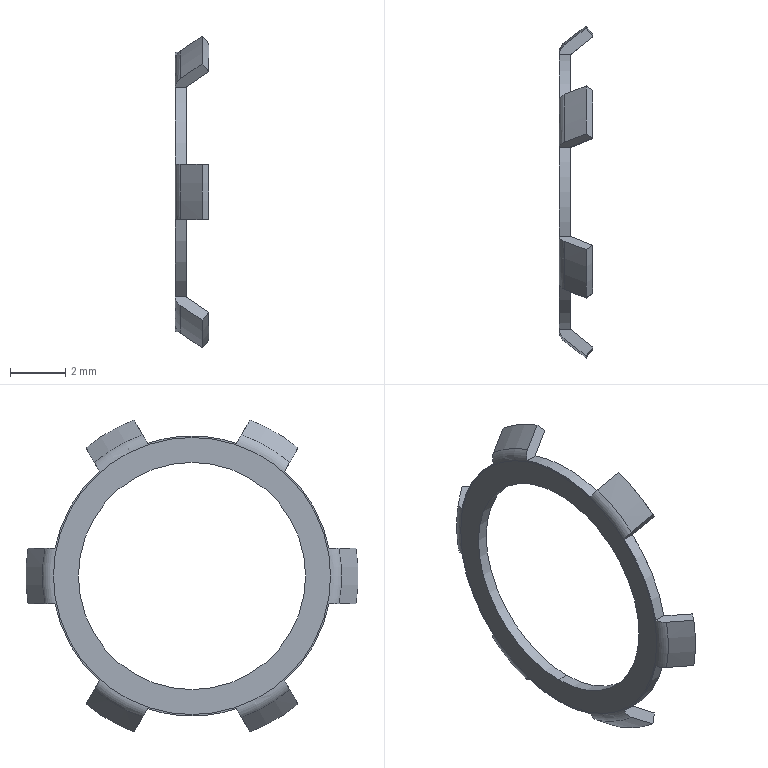Part | STEP file | Outer_ring_gear_2 | 1 solid | 45 faces | box 1.224 x 12 x 11.247 mm | volume 16.794 mm3 | cone 18 | plane 14 | cylinder 9 | torus 4 | commonest cylinder face diameters 10.1 x7 8.2 x2